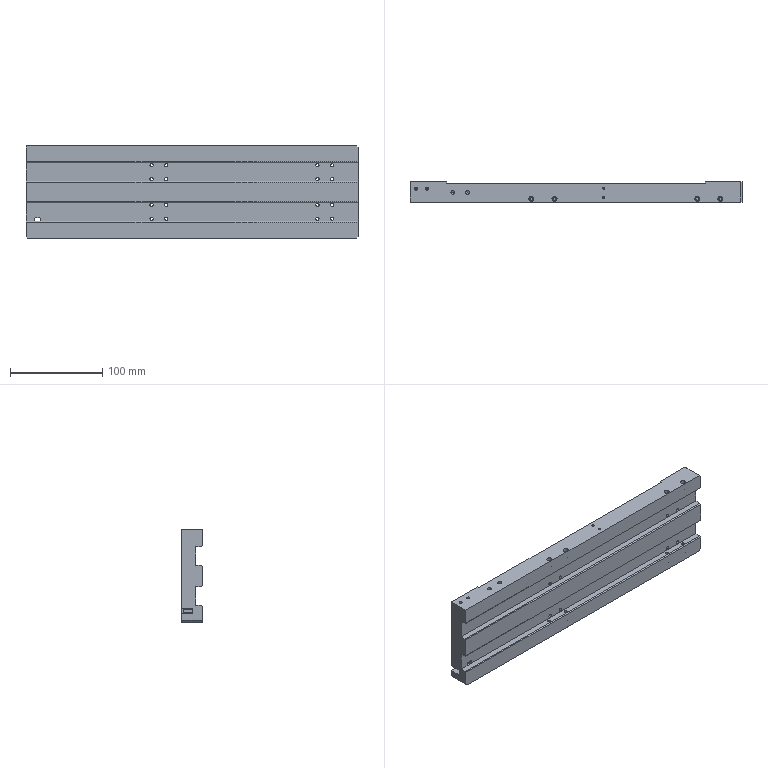Part | SolidWorks | features ICE 9, HoleWzd 7, 3DProfileFeature 5, Chamfer 2, Fillet 2, Extrusion 1, LPattern 1, MirrorPattern 1 | 1 solid | 209 faces | box 360 x 22 x 100 mm | volume 594910 mm3 | cylinder 122 | plane 69 | cone 18 | commonest cylinder face diameters 3.5 x36 7.5 x32 3.3 x20 5.5 x16 4.2 x10 2.5 x4